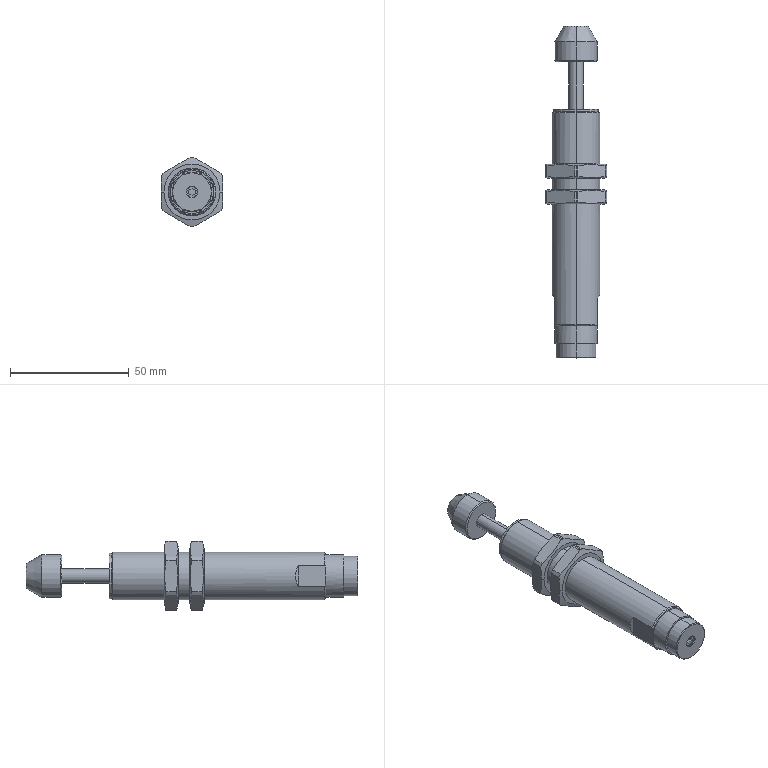Part | SolidWorks | features BaseBody 3 | 3 solids | 100 faces | box 26 x 139.5 x 29.132 mm | volume 38717 mm3 | plane 36 | cylinder 32 | cone 32 | commonest cylinder face diameters 29.132 x14 18 x4 19.188 x4 4.459 x2 6 x2 16.8 x2